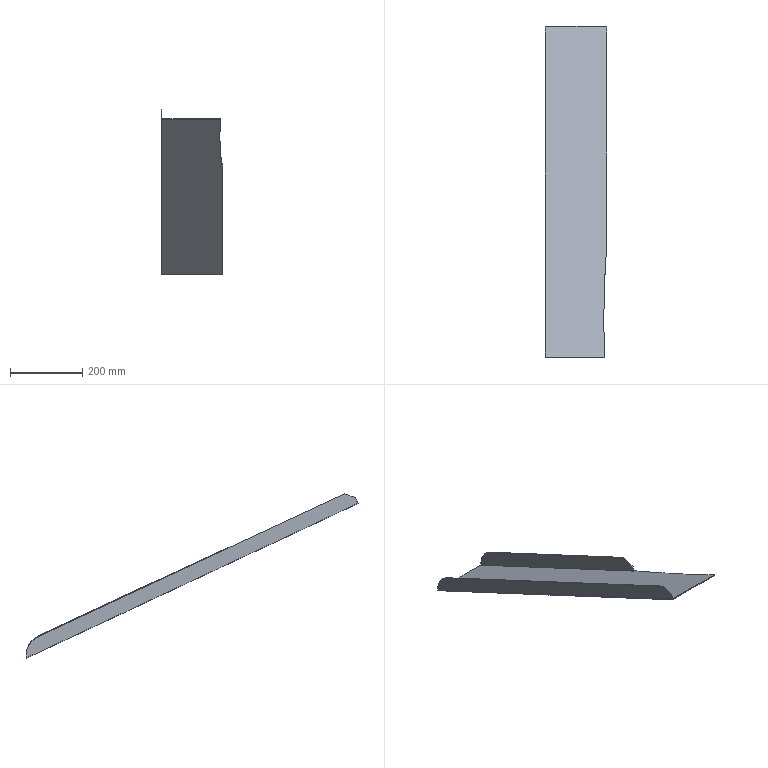Part | NX | features solid 2 | 1 solid | 16 faces | box 171.157 x 921.312 x 456.509 mm | volume 469126 mm3 | plane 13 | cylinder 2 | spline 1 | commonest cylinder face diameters 120 x2
STEP:
#1=CARTESIAN_POINT('',(-1043.,-110.466,-60.636));
#2=VERTEX_POINT('',#1);
#3=CARTESIAN_POINT('',(-1043.,810.,-489.857));
#4=VERTEX_POINT('',#3);
#5=CARTESIAN_POINT('',(-1043.,-181.59,-27.471));
#6=DIRECTION('',(0.,-0.9063,0.4226));
#7=VECTOR('',#6,1000.);
#8=LINE('',#5,#7);
#9=EDGE_CURVE('',#2,#4,#8,.F.);
#10=ORIENTED_EDGE('',*,*,#9,.F.);
#11=CARTESIAN_POINT('',(-880.316,-110.466,-60.636));
#12=VERTEX_POINT('',#11);
#13=CARTESIAN_POINT('',(-1015.,-110.466,-60.636));
#14=DIRECTION('',(-1.,0.,0.));
#15=VECTOR('',#14,1000.);
#16=LINE('',#13,#15);
#17=EDGE_CURVE('',#2,#12,#16,.F.);
#18=ORIENTED_EDGE('',*,*,#17,.T.);
#19=CARTESIAN_POINT('',(-873.944,209.021,-209.616));
#20=VERTEX_POINT('',#19);
#21=CARTESIAN_POINT('',(-880.316,-110.466,-60.636));
#22=CARTESIAN_POINT('',(-881.421,-83.84,-73.052));
#23=CARTESIAN_POINT('',(-882.741,-30.581,-97.887));
#24=CARTESIAN_POINT('',(-882.249,36.029,-128.948));
#25=CARTESIAN_POINT('',(-880.622,89.295,-153.786));
#26=CARTESIAN_POINT('',(-878.685,129.214,-172.401));
#27=CARTESIAN_POINT('',(-876.272,169.116,-191.008));
#28=CARTESIAN_POINT('',(-874.727,195.72,-203.413));
#29=CARTESIAN_POINT('',(-873.944,209.021,-209.616));
#30=B_SPLINE_CURVE_WITH_KNOTS('',3,(#21,#22,#23,#24,#25,#26,#27,#28,#29),.UNSPECIFIED.,.F.,.F.,(4,1,1,1,1,1,4),(1.492,1.58,1.668,1.712,1.757,1.801,1.845),.UNSPECIFIED.);
#31=EDGE_CURVE('',#12,#20,#30,.T.);
#32=ORIENTED_EDGE('',*,*,#31,.T.);
#33=CARTESIAN_POINT('',(-875.843,209.021,-209.616));
#34=VERTEX_POINT('',#33);
#35=CARTESIAN_POINT('',(-1015.,209.021,-209.616));
#36=DIRECTION('',(1.,0.,0.));
#37=VECTOR('',#36,1000.);
#38=LINE('',#35,#37);
#39=EDGE_CURVE('',#20,#34,#38,.F.);
#40=ORIENTED_EDGE('',*,*,#39,.T.);
#41=CARTESIAN_POINT('',(-875.843,810.,-489.857));
#42=VERTEX_POINT('',#41);
#43=CARTESIAN_POINT('',(-875.843,878.67,-521.878));
#44=DIRECTION('',(0.,0.9063,-0.4226));
#45=VECTOR('',#44,1000.);
#46=LINE('',#43,#45);
#47=EDGE_CURVE('',#42,#34,#46,.F.);
#48=ORIENTED_EDGE('',*,*,#47,.F.);
#49=CARTESIAN_POINT('',(-1015.,810.,-489.857));
#50=DIRECTION('',(1.,0.,0.));
#51=VECTOR('',#50,1000.);
#52=LINE('',#49,#51);
#53=EDGE_CURVE('',#42,#4,#52,.F.);
#54=ORIENTED_EDGE('',*,*,#53,.T.);
#55=EDGE_LOOP('',(#10,#18,#32,#40,#48,#54));
#56=FACE_BOUND('',#55,.T.);
#57=CARTESIAN_POINT('',(-1015.,-181.59,-27.471));
#58=DIRECTION('',(0.,0.4226,0.9063));
#59=DIRECTION('',(1.,0.,0.));
#60=AXIS2_PLACEMENT_3D('',#57,#58,#59);
#61=PLANE('',#60);
#62=ADVANCED_FACE('',(#56),#61,.T.);
#63=CARTESIAN_POINT('',(-1045.,810.,-486.152));
#64=VERTEX_POINT('',#63);
#65=CARTESIAN_POINT('',(-1045.,810.,-492.063));
#66=VERTEX_POINT('',#65);
#67=CARTESIAN_POINT('',(-1045.,810.,-18.408));
#68=DIRECTION('',(0.,0.,-1.));
#69=VECTOR('',#68,1000.);
#70=LINE('',#67,#69);
#71=EDGE_CURVE('',#64,#66,#70,.T.);
#72=ORIENTED_EDGE('',*,*,#71,.F.);
#73=CARTESIAN_POINT('',(-1043.,810.,-486.152));
#74=VERTEX_POINT('',#73);
#75=CARTESIAN_POINT('',(-1043.,810.,-486.152));
#76=DIRECTION('',(1.,0.,0.));
#77=VECTOR('',#76,1000.);
#78=LINE('',#75,#77);
#79=EDGE_CURVE('',#64,#74,#78,.T.);
#80=ORIENTED_EDGE('',*,*,#79,.T.);
#81=CARTESIAN_POINT('',(-1043.,810.,-514.935));
#82=DIRECTION('',(0.,0.,1.));
#83=VECTOR('',#82,1000.);
#84=LINE('',#81,#83);
#85=EDGE_CURVE('',#4,#74,#84,.T.);
#86=ORIENTED_EDGE('',*,*,#85,.F.);
#87=ORIENTED_EDGE('',*,*,#53,.F.);
#88=CARTESIAN_POINT('',(-875.843,810.,-483.946));
#89=VERTEX_POINT('',#88);
#90=CARTESIAN_POINT('',(-875.843,810.,-560.));
#91=DIRECTION('',(0.,0.,-1.));
#92=VECTOR('',#91,1000.);
#93=LINE('',#90,#92);
#94=EDGE_CURVE('',#89,#42,#93,.T.);
#95=ORIENTED_EDGE('',*,*,#94,.F.);
#96=CARTESIAN_POINT('',(-873.843,810.,-483.946));
#97=VERTEX_POINT('',#96);
#98=CARTESIAN_POINT('',(1315.,810.,-483.946));
#99=DIRECTION('',(-1.,0.,0.));
#100=VECTOR('',#99,1000.);
#101=LINE('',#98,#100);
#102=EDGE_CURVE('',#89,#97,#101,.F.);
#103=ORIENTED_EDGE('',*,*,#102,.T.);
#104=CARTESIAN_POINT('',(-873.843,810.,-492.063));
#105=VERTEX_POINT('',#104);
#106=CARTESIAN_POINT('',(-873.843,810.,-18.408));
#107=DIRECTION('',(0.,0.,-1.));
#108=VECTOR('',#107,1000.);
#109=LINE('',#106,#108);
#110=EDGE_CURVE('',#97,#105,#109,.T.);
#111=ORIENTED_EDGE('',*,*,#110,.T.);
#112=CARTESIAN_POINT('',(-1015.,810.,-492.063));
#113=DIRECTION('',(1.,0.,0.));
#114=VECTOR('',#113,1000.);
#115=LINE('',#112,#114);
#116=EDGE_CURVE('',#105,#66,#115,.F.);
#117=ORIENTED_EDGE('',*,*,#116,.T.);
#118=EDGE_LOOP('',(#72,#80,#86,#87,#95,#103,#111,#117));
#119=FACE_BOUND('',#118,.T.);
#120=CARTESIAN_POINT('',(1315.,810.,-560.));
#121=DIRECTION('',(0.,-1.,0.));
#122=DIRECTION('',(0.,0.,1.));
#123=AXIS2_PLACEMENT_3D('',#120,#121,#122);
#124=PLANE('',#123);
#125=ADVANCED_FACE('',(#119),#124,.F.);
#126=CARTESIAN_POINT('',(-873.843,214.093,-198.74));
#127=VERTEX_POINT('',#126);
#128=CARTESIAN_POINT('',(-873.843,208.176,-211.428));
#129=VERTEX_POINT('',#128);
#130=CARTESIAN_POINT('',(-873.843,213.248,-200.553));
#131=DIRECTION('',(0.,-0.4226,-0.9063));
#132=VECTOR('',#131,1000.);
#133=LINE('',#130,#132);
#134=EDGE_CURVE('',#127,#129,#133,.T.);
#135=ORIENTED_EDGE('',*,*,#134,.F.);
#136=CARTESIAN_POINT('',(-875.843,214.093,-198.74));
#137=VERTEX_POINT('',#136);
#138=CARTESIAN_POINT('',(-875.843,214.093,-198.74));
#139=DIRECTION('',(-1.,0.,0.));
#140=VECTOR('',#139,1000.);
#141=LINE('',#138,#140);
#142=EDGE_CURVE('',#127,#137,#141,.T.);
#143=ORIENTED_EDGE('',*,*,#142,.T.);
#144=CARTESIAN_POINT('',(-875.843,213.248,-200.553));
#145=DIRECTION('',(0.,0.4226,0.9063));
#146=VECTOR('',#145,1000.);
#147=LINE('',#144,#146);
#148=EDGE_CURVE('',#34,#137,#147,.T.);
#149=ORIENTED_EDGE('',*,*,#148,.F.);
#150=ORIENTED_EDGE('',*,*,#39,.F.);
#151=CARTESIAN_POINT('',(-873.944,208.176,-211.428));
#152=VERTEX_POINT('',#151);
#153=CARTESIAN_POINT('',(-873.944,209.021,-209.616));
#154=CARTESIAN_POINT('',(-873.944,208.74,-210.22));
#155=CARTESIAN_POINT('',(-873.944,208.458,-210.824));
#156=CARTESIAN_POINT('',(-873.944,208.176,-211.428));
#157=B_SPLINE_CURVE_WITH_KNOTS('',3,(#153,#154,#155,#156),.UNSPECIFIED.,.F.,.F.,(4,4),(5.,6.),.UNSPECIFIED.);
#158=EDGE_CURVE('',#20,#152,#157,.T.);
#159=ORIENTED_EDGE('',*,*,#158,.T.);
#160=CARTESIAN_POINT('',(-1015.,208.176,-211.428));
#161=DIRECTION('',(1.,0.,0.));
#162=VECTOR('',#161,1000.);
#163=LINE('',#160,#162);
#164=EDGE_CURVE('',#129,#152,#163,.F.);
#165=ORIENTED_EDGE('',*,*,#164,.F.);
#166=EDGE_LOOP('',(#135,#143,#149,#150,#159,#165));
#167=FACE_BOUND('',#166,.T.);
#168=CARTESIAN_POINT('',(-1015.,213.248,-200.553));
#169=DIRECTION('',(0.,-0.9063,0.4226));
#170=DIRECTION('',(0.,-0.4226,-0.9063));
#171=AXIS2_PLACEMENT_3D('',#168,#169,#170);
#172=PLANE('',#171);
#173=ADVANCED_FACE('',(#167),#172,.T.);
#174=ORIENTED_EDGE('',*,*,#110,.F.);
#175=CARTESIAN_POINT('',(-873.843,775.357,-429.567));
#176=VERTEX_POINT('',#175);
#177=CARTESIAN_POINT('',(-873.843,750.,-483.946));
#178=DIRECTION('',(1.,0.,0.));
#179=DIRECTION('',(0.,0.,-1.));
#180=AXIS2_PLACEMENT_3D('',#177,#178,#179);
#181=CIRCLE('',#180,60.);
#182=EDGE_CURVE('',#97,#176,#181,.T.);
#183=ORIENTED_EDGE('',*,*,#182,.T.);
#184=CARTESIAN_POINT('',(-873.843,251.303,-185.197));
#185=VERTEX_POINT('',#184);
#186=CARTESIAN_POINT('',(-873.843,895.575,-485.626));
#187=DIRECTION('',(0.,-0.9063,0.4226));
#188=VECTOR('',#187,1000.);
#189=LINE('',#186,#188);
#190=EDGE_CURVE('',#176,#185,#189,.T.);
#191=ORIENTED_EDGE('',*,*,#190,.T.);
#192=CARTESIAN_POINT('',(-873.843,-73.614,-303.457));
#193=DIRECTION('',(0.,-0.9397,-0.342));
#194=VECTOR('',#193,1000.);
#195=LINE('',#192,#194);
#196=EDGE_CURVE('',#185,#127,#195,.T.);
#197=ORIENTED_EDGE('',*,*,#196,.T.);
#198=ORIENTED_EDGE('',*,*,#134,.T.);
#199=CARTESIAN_POINT('',(-873.843,-182.435,-29.283));
#200=DIRECTION('',(0.,0.9063,-0.4226));
#201=VECTOR('',#200,1000.);
#202=LINE('',#199,#201);
#203=EDGE_CURVE('',#105,#129,#202,.F.);
#204=ORIENTED_EDGE('',*,*,#203,.F.);
#205=EDGE_LOOP('',(#174,#183,#191,#197,#198,#204));
#206=FACE_BOUND('',#205,.T.);
#207=CARTESIAN_POINT('',(-873.843,-177.364,-18.408));
#208=DIRECTION('',(1.,0.,0.));
#209=DIRECTION('',(0.,-0.08716,-0.9962));
#210=AXIS2_PLACEMENT_3D('',#207,#208,#209);
#211=PLANE('',#210);
#212=ADVANCED_FACE('',(#206),#211,.T.);
#213=CARTESIAN_POINT('',(-1045.,775.357,-431.774));
#214=VERTEX_POINT('',#213);
#215=CARTESIAN_POINT('',(-1045.,-74.339,-35.554));
#216=VERTEX_POINT('',#215);
#217=CARTESIAN_POINT('',(-1045.,895.389,-487.746));
#218=DIRECTION('',(0.,-0.9063,0.4226));
#219=VECTOR('',#218,1000.);
#220=LINE('',#217,#219);
#221=EDGE_CURVE('',#214,#216,#220,.T.);
#222=ORIENTED_EDGE('',*,*,#221,.F.);
#223=CARTESIAN_POINT('',(-1045.,750.,-486.152));
#224=DIRECTION('',(1.,0.,0.));
#225=DIRECTION('',(0.,0.,-1.));
#226=AXIS2_PLACEMENT_3D('',#223,#224,#225);
#227=CIRCLE('',#226,60.);
#228=EDGE_CURVE('',#214,#64,#227,.F.);
#229=ORIENTED_EDGE('',*,*,#228,.T.);
#230=ORIENTED_EDGE('',*,*,#71,.T.);
#231=CARTESIAN_POINT('',(-1045.,-111.312,-62.449));
#232=VERTEX_POINT('',#231);
#233=CARTESIAN_POINT('',(-1045.,-182.435,-29.283));
#234=DIRECTION('',(0.,0.9063,-0.4226));
#235=VECTOR('',#234,1000.);
#236=LINE('',#233,#235);
#237=EDGE_CURVE('',#66,#232,#236,.F.);
#238=ORIENTED_EDGE('',*,*,#237,.T.);
#239=CARTESIAN_POINT('',(-1045.,-103.765,-46.264));
#240=VERTEX_POINT('',#239);
#241=CARTESIAN_POINT('',(-1045.,-106.24,-51.573));
#242=DIRECTION('',(0.,-0.4226,-0.9063));
#243=VECTOR('',#242,1000.);
#244=LINE('',#241,#243);
#245=EDGE_CURVE('',#240,#232,#244,.T.);
#246=ORIENTED_EDGE('',*,*,#245,.F.);
#247=CARTESIAN_POINT('',(-1045.,-83.736,-38.974));
#248=DIRECTION('',(0.,-0.9397,-0.342));
#249=VECTOR('',#248,1000.);
#250=LINE('',#247,#249);
#251=EDGE_CURVE('',#240,#216,#250,.F.);
#252=ORIENTED_EDGE('',*,*,#251,.T.);
#253=EDGE_LOOP('',(#222,#229,#230,#238,#246,#252));
#254=FACE_BOUND('',#253,.T.);
#255=CARTESIAN_POINT('',(-1045.,-177.364,-18.408));
#256=DIRECTION('',(1.,0.,0.));
#257=DIRECTION('',(0.,-0.08716,-0.9962));
#258=AXIS2_PLACEMENT_3D('',#255,#256,#257);
#259=PLANE('',#258);
#260=ADVANCED_FACE('',(#254),#259,.F.);
#261=ORIENTED_EDGE('',*,*,#17,.F.);
#262=CARTESIAN_POINT('',(-1043.,-103.765,-46.264));
#263=VERTEX_POINT('',#262);
#264=CARTESIAN_POINT('',(-1043.,-106.24,-51.573));
#265=DIRECTION('',(0.,0.4226,0.9063));
#266=VECTOR('',#265,1000.);
#267=LINE('',#264,#266);
#268=EDGE_CURVE('',#2,#263,#267,.T.);
#269=ORIENTED_EDGE('',*,*,#268,.T.);
#270=CARTESIAN_POINT('',(-1045.,-103.765,-46.264));
#271=DIRECTION('',(1.,0.,0.));
#272=VECTOR('',#271,1000.);
#273=LINE('',#270,#272);
#274=EDGE_CURVE('',#263,#240,#273,.F.);
#275=ORIENTED_EDGE('',*,*,#274,.T.);
#276=ORIENTED_EDGE('',*,*,#245,.T.);
#277=CARTESIAN_POINT('',(-880.316,-111.312,-62.449));
#278=VERTEX_POINT('',#277);
#279=CARTESIAN_POINT('',(-1015.,-111.312,-62.449));
#280=DIRECTION('',(-1.,0.,0.));
#281=VECTOR('',#280,1000.);
#282=LINE('',#279,#281);
#283=EDGE_CURVE('',#232,#278,#282,.F.);
#284=ORIENTED_EDGE('',*,*,#283,.T.);
#285=CARTESIAN_POINT('',(-880.316,-108.776,-57.011));
#286=DIRECTION('',(0.,-0.4226,-0.9063));
#287=VECTOR('',#286,1000.);
#288=LINE('',#285,#287);
#289=EDGE_CURVE('',#12,#278,#288,.T.);
#290=ORIENTED_EDGE('',*,*,#289,.F.);
#291=EDGE_LOOP('',(#261,#269,#275,#276,#284,#290));
#292=FACE_BOUND('',#291,.T.);
#293=CARTESIAN_POINT('',(-1015.,-106.24,-51.573));
#294=DIRECTION('',(0.,0.9063,-0.4226));
#295=DIRECTION('',(0.,0.4226,0.9063));
#296=AXIS2_PLACEMENT_3D('',#293,#294,#295);
#297=PLANE('',#296);
#298=ADVANCED_FACE('',(#292),#297,.F.);
#299=CARTESIAN_POINT('',(-880.316,-111.312,-62.449));
#300=CARTESIAN_POINT('',(-881.421,-84.685,-74.865));
#301=CARTESIAN_POINT('',(-882.741,-31.426,-99.7));
#302=CARTESIAN_POINT('',(-882.249,35.184,-130.761));
#303=CARTESIAN_POINT('',(-880.622,88.45,-155.599));
#304=CARTESIAN_POINT('',(-878.685,128.369,-174.214));
#305=CARTESIAN_POINT('',(-876.272,168.271,-192.82));
#306=CARTESIAN_POINT('',(-874.727,194.875,-205.226));
#307=CARTESIAN_POINT('',(-873.944,208.176,-211.428));
#308=B_SPLINE_CURVE_WITH_KNOTS('',3,(#299,#300,#301,#302,#303,#304,#305,#306,#307),.UNSPECIFIED.,.F.,.F.,(4,1,1,1,1,1,4),(1.492,1.58,1.668,1.712,1.757,1.801,1.845),.UNSPECIFIED.);
#309=EDGE_CURVE('',#278,#152,#308,.T.);
#310=ORIENTED_EDGE('',*,*,#309,.T.);
#311=ORIENTED_EDGE('',*,*,#158,.F.);
#312=ORIENTED_EDGE('',*,*,#31,.F.);
#313=ORIENTED_EDGE('',*,*,#289,.T.);
#314=EDGE_LOOP('',(#310,#311,#312,#313));
#315=FACE_BOUND('',#314,.T.);
#316=CARTESIAN_POINT('',(-880.316,-110.466,-60.636));
#317=CARTESIAN_POINT('',(-880.316,-111.312,-62.449));
#318=CARTESIAN_POINT('',(-880.862,-97.299,-66.776));
#319=CARTESIAN_POINT('',(-880.862,-98.144,-68.589));
#320=CARTESIAN_POINT('',(-881.741,-70.879,-79.096));
#321=CARTESIAN_POINT('',(-881.741,-71.725,-80.908));
#322=CARTESIAN_POINT('',(-882.416,-30.996,-97.694));
#323=CARTESIAN_POINT('',(-882.416,-31.841,-99.507));
#324=CARTESIAN_POINT('',(-882.444,2.452,-113.291));
#325=CARTESIAN_POINT('',(-882.444,1.607,-115.103));
#326=CARTESIAN_POINT('',(-882.146,29.339,-125.828));
#327=CARTESIAN_POINT('',(-882.146,28.494,-127.641));
#328=CARTESIAN_POINT('',(-881.762,49.561,-135.258));
#329=CARTESIAN_POINT('',(-881.762,48.716,-137.071));
#330=CARTESIAN_POINT('',(-881.31,66.286,-143.057));
#331=CARTESIAN_POINT('',(-881.31,65.44,-144.869));
#332=CARTESIAN_POINT('',(-880.868,79.62,-149.275));
#333=CARTESIAN_POINT('',(-880.868,78.774,-151.087));
#334=CARTESIAN_POINT('',(-880.497,89.592,-153.925));
#335=CARTESIAN_POINT('',(-880.497,88.747,-155.738));
#336=CARTESIAN_POINT('',(-880.155,97.881,-157.79));
#337=CARTESIAN_POINT('',(-880.155,97.036,-159.603));
#338=CARTESIAN_POINT('',(-879.861,104.499,-160.876));
#339=CARTESIAN_POINT('',(-879.861,103.654,-162.689));
#340=CARTESIAN_POINT('',(-879.631,109.455,-163.187));
#341=CARTESIAN_POINT('',(-879.631,108.61,-165.));
#342=CARTESIAN_POINT('',(-879.431,113.58,-165.111));
#343=CARTESIAN_POINT('',(-879.431,112.735,-166.923));
#344=CARTESIAN_POINT('',(-879.266,116.877,-166.648));
#345=CARTESIAN_POINT('',(-879.266,116.031,-168.461));
#346=CARTESIAN_POINT('',(-879.161,118.936,-167.608));
#347=CARTESIAN_POINT('',(-879.161,118.091,-169.421));
#348=CARTESIAN_POINT('',(-879.075,120.582,-168.376));
#349=CARTESIAN_POINT('',(-879.075,119.737,-170.188));
#350=CARTESIAN_POINT('',(-879.011,121.817,-168.952));
#351=CARTESIAN_POINT('',(-879.011,120.972,-170.764));
#352=CARTESIAN_POINT('',(-878.956,122.842,-169.43));
#353=CARTESIAN_POINT('',(-878.956,121.997,-171.242));
#354=CARTESIAN_POINT('',(-878.912,123.671,-169.816));
#355=CARTESIAN_POINT('',(-878.912,122.826,-171.629));
#356=CARTESIAN_POINT('',(-878.886,124.168,-170.048));
#357=CARTESIAN_POINT('',(-878.886,123.323,-171.861));
#358=CARTESIAN_POINT('',(-878.865,124.559,-170.23));
#359=CARTESIAN_POINT('',(-878.865,123.713,-172.043));
#360=CARTESIAN_POINT('',(-878.856,124.715,-170.303));
#361=CARTESIAN_POINT('',(-878.856,123.869,-172.115));
#362=CARTESIAN_POINT('',(-878.855,124.738,-170.314));
#363=CARTESIAN_POINT('',(-878.855,123.893,-172.127));
#364=CARTESIAN_POINT('',(-878.851,124.815,-170.349));
#365=CARTESIAN_POINT('',(-878.851,123.97,-172.162));
#366=CARTESIAN_POINT('',(-878.843,124.964,-170.419));
#367=CARTESIAN_POINT('',(-878.843,124.119,-172.232));
#368=CARTESIAN_POINT('',(-878.823,125.328,-170.589));
#369=CARTESIAN_POINT('',(-878.823,124.483,-172.401));
#370=CARTESIAN_POINT('',(-878.789,125.944,-170.876));
#371=CARTESIAN_POINT('',(-878.789,125.098,-172.688));
#372=CARTESIAN_POINT('',(-878.741,126.801,-171.276));
#373=CARTESIAN_POINT('',(-878.741,125.956,-173.088));
#374=CARTESIAN_POINT('',(-878.669,128.091,-171.877));
#375=CARTESIAN_POINT('',(-878.669,127.246,-173.69));
#376=CARTESIAN_POINT('',(-878.562,129.986,-172.761));
#377=CARTESIAN_POINT('',(-878.562,129.14,-174.573));
#378=CARTESIAN_POINT('',(-878.406,132.707,-174.03));
#379=CARTESIAN_POINT('',(-878.406,131.862,-175.843));
#380=CARTESIAN_POINT('',(-878.163,136.935,-176.001));
#381=CARTESIAN_POINT('',(-878.163,136.09,-177.814));
#382=CARTESIAN_POINT('',(-877.644,145.905,-180.184));
#383=CARTESIAN_POINT('',(-877.644,145.06,-181.997));
#384=CARTESIAN_POINT('',(-876.433,166.67,-189.867));
#385=CARTESIAN_POINT('',(-876.433,165.825,-191.679));
#386=CARTESIAN_POINT('',(-874.977,191.456,-201.425));
#387=CARTESIAN_POINT('',(-874.977,190.611,-203.237));
#388=CARTESIAN_POINT('',(-873.944,209.021,-209.616));
#389=CARTESIAN_POINT('',(-873.944,208.176,-211.428));
#390=B_SPLINE_SURFACE_WITH_KNOTS('',3,1,((#316,#317),(#318,#319),(#320,#321),(#322,#323),(#324,#325),(#326,#327),(#328,#329),(#330,#331),(#332,#333),(#334,#335),(#336,#337),(#338,#339),(#340,#341),(#342,#343),(#344,#345),(#346,#347),(#348,#349),(#350,#351),(#352,#353),(#354,#355),(#356,#357),(#358,#359),(#360,#361),(#362,#363),(#364,#365),(#366,#367),(#368,#369),(#370,#371),(#372,#373),(#374,#375),(#376,#377),(#378,#379),(#380,#381),(#382,#383),(#384,#385),(#386,#387),(#388,#389)),.UNSPECIFIED.,.F.,.F.,.F.,(4,1,1,1,1,1,1,1,1,1,1,1,1,1,1,1,1,1,1,1,1,1,1,1,1,1,1,1,1,1,1,1,1,1,4),(2,2),(0.05432,0.1725,0.2907,0.409,0.4681,0.5272,0.5863,0.6158,0.6454,0.6749,0.6897,0.7045,0.7193,0.7266,0.734,0.7377,0.7414,0.7451,0.747,0.7488,0.7497,0.7502,0.7507,0.7516,0.7525,0.7562,0.7636,0.771,0.7784,0.7931,0.8079,0.8227,0.8522,0.9113,1.),(0.,1.),.UNSPECIFIED.);
#391=ADVANCED_FACE('',(#315),#390,.F.);
#392=ORIENTED_EDGE('',*,*,#237,.F.);
#393=ORIENTED_EDGE('',*,*,#116,.F.);
#394=ORIENTED_EDGE('',*,*,#203,.T.);
#395=ORIENTED_EDGE('',*,*,#164,.T.);
#396=ORIENTED_EDGE('',*,*,#309,.F.);
#397=ORIENTED_EDGE('',*,*,#283,.F.);
#398=EDGE_LOOP('',(#392,#393,#394,#395,#396,#397));
#399=FACE_BOUND('',#398,.T.);
#400=CARTESIAN_POINT('',(-1015.,-182.435,-29.283));
#401=DIRECTION('',(0.,0.4226,0.9063));
#402=DIRECTION('',(1.,0.,0.));
#403=AXIS2_PLACEMENT_3D('',#400,#401,#402);
#404=PLANE('',#403);
#405=ADVANCED_FACE('',(#399),#404,.F.);
#406=ORIENTED_EDGE('',*,*,#190,.F.);
#407=CARTESIAN_POINT('',(-875.843,775.357,-429.567));
#408=VERTEX_POINT('',#407);
#409=CARTESIAN_POINT('',(-873.843,775.357,-429.567));
#410=DIRECTION('',(-1.,0.,0.));
#411=VECTOR('',#410,1000.);
#412=LINE('',#409,#411);
#413=EDGE_CURVE('',#176,#408,#412,.T.);
#414=ORIENTED_EDGE('',*,*,#413,.T.);
#415=CARTESIAN_POINT('',(-875.843,251.303,-185.197));
#416=VERTEX_POINT('',#415);
#417=CARTESIAN_POINT('',(-875.843,895.575,-485.626));
#418=DIRECTION('',(0.,-0.9063,0.4226));
#419=VECTOR('',#418,1000.);
#420=LINE('',#417,#419);
#421=EDGE_CURVE('',#408,#416,#420,.T.);
#422=ORIENTED_EDGE('',*,*,#421,.T.);
#423=CARTESIAN_POINT('',(-873.843,251.303,-185.197));
#424=DIRECTION('',(1.,0.,0.));
#425=VECTOR('',#424,1000.);
#426=LINE('',#423,#425);
#427=EDGE_CURVE('',#416,#185,#426,.T.);
#428=ORIENTED_EDGE('',*,*,#427,.T.);
#429=EDGE_LOOP('',(#406,#414,#422,#428));
#430=FACE_BOUND('',#429,.T.);
#431=CARTESIAN_POINT('',(-873.843,895.575,-485.626));
#432=DIRECTION('',(0.,-0.4226,-0.9063));
#433=DIRECTION('',(0.,-0.9063,0.4226));
#434=AXIS2_PLACEMENT_3D('',#431,#432,#433);
#435=PLANE('',#434);
#436=ADVANCED_FACE('',(#430),#435,.F.);
#437=ORIENTED_EDGE('',*,*,#421,.F.);
#438=CARTESIAN_POINT('',(-875.843,750.,-483.946));
#439=DIRECTION('',(-1.,0.,0.));
#440=DIRECTION('',(0.,0.,1.));
#441=AXIS2_PLACEMENT_3D('',#438,#439,#440);
#442=CIRCLE('',#441,60.);
#443=EDGE_CURVE('',#408,#89,#442,.T.);
#444=ORIENTED_EDGE('',*,*,#443,.T.);
#445=ORIENTED_EDGE('',*,*,#94,.T.);
#446=ORIENTED_EDGE('',*,*,#47,.T.);
#447=ORIENTED_EDGE('',*,*,#148,.T.);
#448=CARTESIAN_POINT('',(-875.843,703.719,-20.531));
#449=DIRECTION('',(0.,0.9397,0.342));
#450=VECTOR('',#449,1000.);
#451=LINE('',#448,#450);
#452=EDGE_CURVE('',#137,#416,#451,.T.);
#453=ORIENTED_EDGE('',*,*,#452,.T.);
#454=EDGE_LOOP('',(#437,#444,#445,#446,#447,#453));
#455=FACE_BOUND('',#454,.T.);
#456=CARTESIAN_POINT('',(-875.843,882.896,-512.815));
#457=DIRECTION('',(-1.,0.,0.));
#458=DIRECTION('',(0.,0.08716,0.9962));
#459=AXIS2_PLACEMENT_3D('',#456,#457,#458);
#460=PLANE('',#459);
#461=ADVANCED_FACE('',(#455),#460,.T.);
#462=ORIENTED_EDGE('',*,*,#85,.T.);
#463=CARTESIAN_POINT('',(-1043.,775.357,-431.774));
#464=VERTEX_POINT('',#463);
#465=CARTESIAN_POINT('',(-1043.,750.,-486.152));
#466=DIRECTION('',(-1.,0.,0.));
#467=DIRECTION('',(0.,0.,1.));
#468=AXIS2_PLACEMENT_3D('',#465,#466,#467);
#469=CIRCLE('',#468,60.);
#470=EDGE_CURVE('',#74,#464,#469,.F.);
#471=ORIENTED_EDGE('',*,*,#470,.T.);
#472=CARTESIAN_POINT('',(-1043.,-74.339,-35.554));
#473=VERTEX_POINT('',#472);
#474=CARTESIAN_POINT('',(-1043.,895.389,-487.746));
#475=DIRECTION('',(0.,-0.9063,0.4226));
#476=VECTOR('',#475,1000.);
#477=LINE('',#474,#476);
#478=EDGE_CURVE('',#464,#473,#477,.T.);
#479=ORIENTED_EDGE('',*,*,#478,.T.);
#480=CARTESIAN_POINT('',(-1043.,-83.736,-38.974));
#481=DIRECTION('',(0.,0.9397,0.342));
#482=VECTOR('',#481,1000.);
#483=LINE('',#480,#482);
#484=EDGE_CURVE('',#473,#263,#483,.F.);
#485=ORIENTED_EDGE('',*,*,#484,.T.);
#486=ORIENTED_EDGE('',*,*,#268,.F.);
#487=ORIENTED_EDGE('',*,*,#9,.T.);
#488=EDGE_LOOP('',(#462,#471,#479,#485,#486,#487));
#489=FACE_BOUND('',#488,.T.);
#490=CARTESIAN_POINT('',(-1043.,882.711,-514.935));
#491=DIRECTION('',(-1.,0.,0.));
#492=DIRECTION('',(0.,0.08716,0.9962));
#493=AXIS2_PLACEMENT_3D('',#490,#491,#492);
#494=PLANE('',#493);
#495=ADVANCED_FACE('',(#489),#494,.F.);
#496=ORIENTED_EDGE('',*,*,#478,.F.);
#497=CARTESIAN_POINT('',(-1045.,775.357,-431.774));
#498=DIRECTION('',(-1.,0.,0.));
#499=VECTOR('',#498,1000.);
#500=LINE('',#497,#499);
#501=EDGE_CURVE('',#464,#214,#500,.T.);
#502=ORIENTED_EDGE('',*,*,#501,.T.);
#503=ORIENTED_EDGE('',*,*,#221,.T.);
#504=CARTESIAN_POINT('',(-1045.,-74.339,-35.554));
#505=DIRECTION('',(1.,0.,0.));
#506=VECTOR('',#505,1000.);
#507=LINE('',#504,#506);
#508=EDGE_CURVE('',#216,#473,#507,.T.);
#509=ORIENTED_EDGE('',*,*,#508,.T.);
#510=EDGE_LOOP('',(#496,#502,#503,#509));
#511=FACE_BOUND('',#510,.T.);
#512=CARTESIAN_POINT('',(-1045.,895.389,-487.746));
#513=DIRECTION('',(0.,-0.4226,-0.9063));
#514=DIRECTION('',(0.,-0.9063,0.4226));
#515=AXIS2_PLACEMENT_3D('',#512,#513,#514);
#516=PLANE('',#515);
#517=ADVANCED_FACE('',(#511),#516,.F.);
#518=ORIENTED_EDGE('',*,*,#251,.F.);
#519=ORIENTED_EDGE('',*,*,#274,.F.);
#520=ORIENTED_EDGE('',*,*,#484,.F.);
#521=ORIENTED_EDGE('',*,*,#508,.F.);
#522=EDGE_LOOP('',(#518,#519,#520,#521));
#523=FACE_BOUND('',#522,.T.);
#524=CARTESIAN_POINT('',(-1045.,-83.736,-38.974));
#525=DIRECTION('',(0.,0.342,-0.9397));
#526=DIRECTION('',(0.,0.9397,0.342));
#527=AXIS2_PLACEMENT_3D('',#524,#525,#526);
#528=PLANE('',#527);
#529=ADVANCED_FACE('',(#523),#528,.F.);
#530=ORIENTED_EDGE('',*,*,#196,.F.);
#531=ORIENTED_EDGE('',*,*,#427,.F.);
#532=ORIENTED_EDGE('',*,*,#452,.F.);
#533=ORIENTED_EDGE('',*,*,#142,.F.);
#534=EDGE_LOOP('',(#530,#531,#532,#533));
#535=FACE_BOUND('',#534,.T.);
#536=CARTESIAN_POINT('',(-1015.,214.093,-198.74));
#537=DIRECTION('',(0.,-0.342,0.9397));
#538=DIRECTION('',(0.,-0.9397,-0.342));
#539=AXIS2_PLACEMENT_3D('',#536,#537,#538);
#540=PLANE('',#539);
#541=ADVANCED_FACE('',(#535),#540,.T.);
#542=ORIENTED_EDGE('',*,*,#182,.F.);
#543=ORIENTED_EDGE('',*,*,#102,.F.);
#544=ORIENTED_EDGE('',*,*,#443,.F.);
#545=ORIENTED_EDGE('',*,*,#413,.F.);
#546=EDGE_LOOP('',(#542,#543,#544,#545));
#547=FACE_BOUND('',#546,.T.);
#548=CARTESIAN_POINT('',(-873.843,750.,-483.946));
#549=DIRECTION('',(-1.,0.,0.));
#550=DIRECTION('',(0.,0.,1.));
#551=AXIS2_PLACEMENT_3D('',#548,#549,#550);
#552=CYLINDRICAL_SURFACE('',#551,60.);
#553=ADVANCED_FACE('',(#547),#552,.T.);
#554=ORIENTED_EDGE('',*,*,#470,.F.);
#555=ORIENTED_EDGE('',*,*,#79,.F.);
#556=ORIENTED_EDGE('',*,*,#228,.F.);
#557=ORIENTED_EDGE('',*,*,#501,.F.);
#558=EDGE_LOOP('',(#554,#555,#556,#557));
#559=FACE_BOUND('',#558,.T.);
#560=CARTESIAN_POINT('',(-1045.,750.,-486.152));
#561=DIRECTION('',(-1.,0.,0.));
#562=DIRECTION('',(0.,0.,1.));
#563=AXIS2_PLACEMENT_3D('',#560,#561,#562);
#564=CYLINDRICAL_SURFACE('',#563,60.);
#565=ADVANCED_FACE('',(#559),#564,.T.);
#566=CLOSED_SHELL('',(#62,#125,#173,#212,#260,#298,#391,#405,#436,#461,#495,#517,#529,#541,#553,#565));
#567=MANIFOLD_SOLID_BREP('',#566);
#568=(LENGTH_UNIT()NAMED_UNIT(*)SI_UNIT(.MILLI.,.METRE.));
#569=UNCERTAINTY_MEASURE_WITH_UNIT(LENGTH_MEASURE(0.0508),#568,'','');
#570=(NAMED_UNIT(*)PLANE_ANGLE_UNIT()SI_UNIT($,.RADIAN.));
#571=(NAMED_UNIT(*)SI_UNIT($,.STERADIAN.)SOLID_ANGLE_UNIT());
#572=(GEOMETRIC_REPRESENTATION_CONTEXT(3)GLOBAL_UNCERTAINTY_ASSIGNED_CONTEXT((#569))GLOBAL_UNIT_ASSIGNED_CONTEXT((#568,#570,#571))REPRESENTATION_CONTEXT('',''));
#573=ADVANCED_BREP_SHAPE_REPRESENTATION('',(#567),#572);